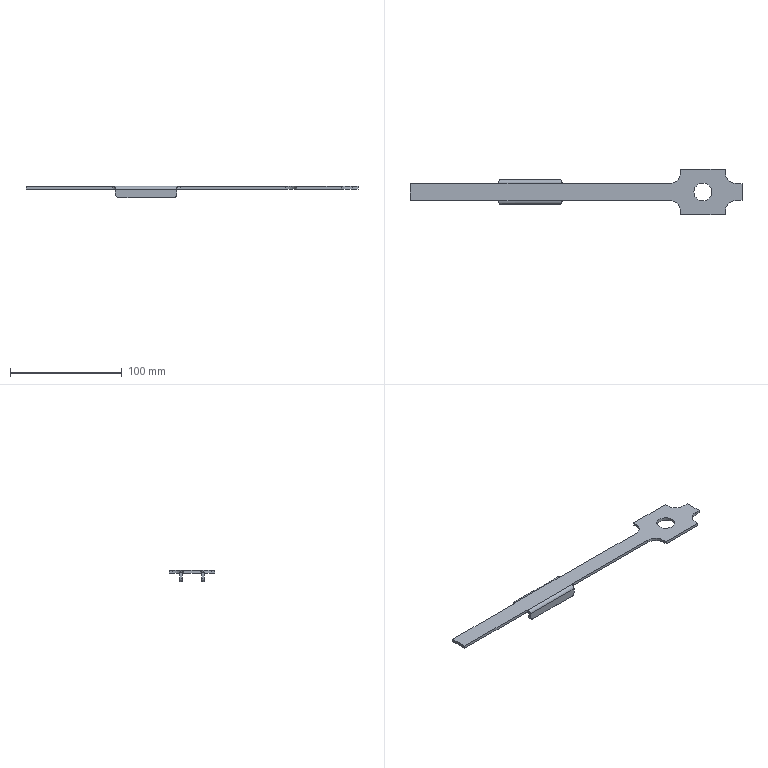Part | STEP file | lll_id1230_x_t | 1 solid | 57 faces | box 297 x 41 x 10 mm | volume 16253 mm3 | plane 32 | cylinder 25 | commonest cylinder face diameters 6 x18 20 x4 1 x2 16.1 x1